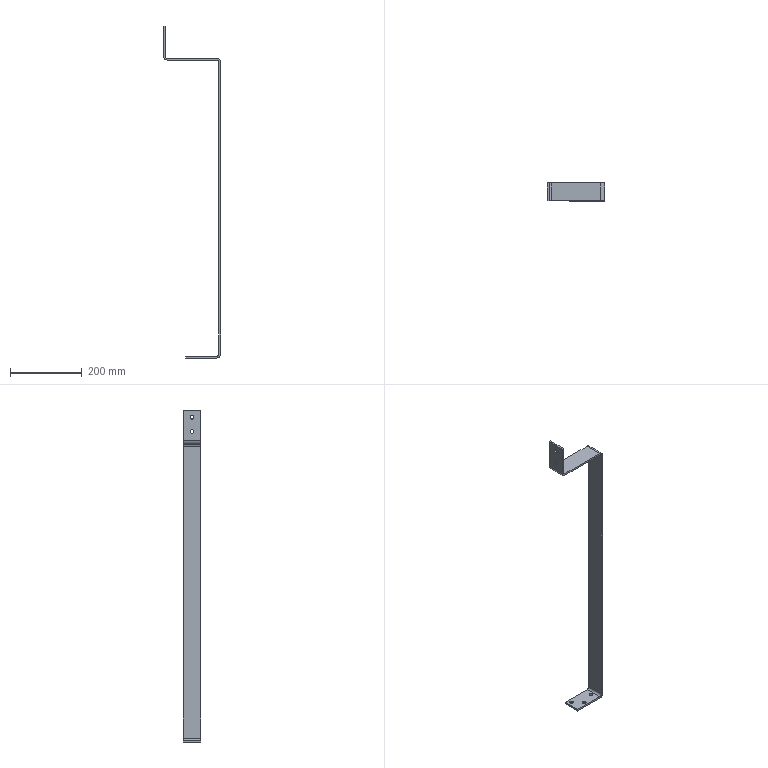Part | SolidWorks | features BaseBody 1 | 1 solid | 28 faces | box 160 x 50 x 926 mm | volume 288422 mm3 | cylinder 16 | plane 12 | commonest cylinder face diameters 11 x8 12 x3 22 x3 10.6 x2
STEP:
#1=CARTESIAN_POINT('',(787.946,-3577.473,1065.971));
#2=VERTEX_POINT('',#1);
#3=CARTESIAN_POINT('',(787.946,-3577.473,1076.971));
#4=VERTEX_POINT('',#3);
#5=CARTESIAN_POINT('',(787.946,-3577.473,1071.471));
#6=DIRECTION('',(-1.,0.,0.));
#7=DIRECTION('',(0.,0.,1.));
#8=AXIS2_PLACEMENT_3D('',#5,#6,#7);
#9=CIRCLE('',#8,5.5);
#10=EDGE_CURVE('',#2,#4,#9,.T.);
#11=ORIENTED_EDGE('',*,*,#10,.F.);
#12=CARTESIAN_POINT('',(782.946,-3577.473,1065.971));
#13=VERTEX_POINT('',#12);
#14=CARTESIAN_POINT('',(781.319,-3577.473,1065.971));
#15=DIRECTION('',(-1.,0.,0.));
#16=VECTOR('',#15,1000.);
#17=LINE('',#14,#16);
#18=EDGE_CURVE('',#2,#13,#17,.T.);
#19=ORIENTED_EDGE('',*,*,#18,.T.);
#20=CARTESIAN_POINT('',(782.946,-3577.473,1076.971));
#21=VERTEX_POINT('',#20);
#22=CARTESIAN_POINT('',(782.946,-3577.473,1071.471));
#23=DIRECTION('',(1.,0.,0.));
#24=DIRECTION('',(0.,0.,1.));
#25=AXIS2_PLACEMENT_3D('',#22,#23,#24);
#26=CIRCLE('',#25,5.5);
#27=EDGE_CURVE('',#21,#13,#26,.T.);
#28=ORIENTED_EDGE('',*,*,#27,.F.);
#29=CARTESIAN_POINT('',(781.319,-3577.473,1076.971));
#30=DIRECTION('',(-1.,0.,0.));
#31=VECTOR('',#30,1000.);
#32=LINE('',#29,#31);
#33=EDGE_CURVE('',#4,#21,#32,.T.);
#34=ORIENTED_EDGE('',*,*,#33,.F.);
#35=EDGE_LOOP('',(#11,#19,#28,#34));
#36=FACE_OUTER_BOUND('',#35,.T.);
#37=CARTESIAN_POINT('',(781.319,-3577.473,1071.471));
#38=DIRECTION('',(-1.,0.,0.));
#39=DIRECTION('',(0.,0.,1.));
#40=AXIS2_PLACEMENT_3D('',#37,#38,#39);
#41=CYLINDRICAL_SURFACE('',#40,5.5);
#42=ADVANCED_FACE('',(#36),#41,.F.);
#43=CARTESIAN_POINT('',(787.946,-3577.473,1025.971));
#44=VERTEX_POINT('',#43);
#45=CARTESIAN_POINT('',(787.946,-3577.473,1036.971));
#46=VERTEX_POINT('',#45);
#47=CARTESIAN_POINT('',(787.946,-3577.473,1031.471));
#48=DIRECTION('',(-1.,0.,0.));
#49=DIRECTION('',(0.,0.,1.));
#50=AXIS2_PLACEMENT_3D('',#47,#48,#49);
#51=CIRCLE('',#50,5.5);
#52=EDGE_CURVE('',#44,#46,#51,.T.);
#53=ORIENTED_EDGE('',*,*,#52,.F.);
#54=CARTESIAN_POINT('',(782.946,-3577.473,1025.971));
#55=VERTEX_POINT('',#54);
#56=CARTESIAN_POINT('',(781.319,-3577.473,1025.971));
#57=DIRECTION('',(-1.,0.,0.));
#58=VECTOR('',#57,1000.);
#59=LINE('',#56,#58);
#60=EDGE_CURVE('',#44,#55,#59,.T.);
#61=ORIENTED_EDGE('',*,*,#60,.T.);
#62=CARTESIAN_POINT('',(782.946,-3577.473,1036.971));
#63=VERTEX_POINT('',#62);
#64=CARTESIAN_POINT('',(782.946,-3577.473,1031.471));
#65=DIRECTION('',(1.,0.,0.));
#66=DIRECTION('',(0.,0.,1.));
#67=AXIS2_PLACEMENT_3D('',#64,#65,#66);
#68=CIRCLE('',#67,5.5);
#69=EDGE_CURVE('',#63,#55,#68,.T.);
#70=ORIENTED_EDGE('',*,*,#69,.F.);
#71=CARTESIAN_POINT('',(781.319,-3577.473,1036.971));
#72=DIRECTION('',(-1.,0.,0.));
#73=VECTOR('',#72,1000.);
#74=LINE('',#71,#73);
#75=EDGE_CURVE('',#46,#63,#74,.T.);
#76=ORIENTED_EDGE('',*,*,#75,.F.);
#77=EDGE_LOOP('',(#53,#61,#70,#76));
#78=FACE_OUTER_BOUND('',#77,.T.);
#79=CARTESIAN_POINT('',(781.319,-3577.473,1031.471));
#80=DIRECTION('',(-1.,0.,0.));
#81=DIRECTION('',(0.,0.,1.));
#82=AXIS2_PLACEMENT_3D('',#79,#80,#81);
#83=CYLINDRICAL_SURFACE('',#82,5.5);
#84=ADVANCED_FACE('',(#78),#83,.F.);
#85=CARTESIAN_POINT('',(916.646,-3577.473,165.471));
#86=VERTEX_POINT('',#85);
#87=CARTESIAN_POINT('',(927.246,-3577.473,165.471));
#88=VERTEX_POINT('',#87);
#89=CARTESIAN_POINT('',(921.946,-3577.473,165.471));
#90=DIRECTION('',(0.,0.,1.));
#91=DIRECTION('',(1.,0.,0.));
#92=AXIS2_PLACEMENT_3D('',#89,#90,#91);
#93=CIRCLE('',#92,5.3);
#94=EDGE_CURVE('',#86,#88,#93,.T.);
#95=ORIENTED_EDGE('',*,*,#94,.F.);
#96=CARTESIAN_POINT('',(916.646,-3577.473,170.471));
#97=VERTEX_POINT('',#96);
#98=CARTESIAN_POINT('',(916.646,-3577.473,155.54));
#99=DIRECTION('',(0.,0.,1.));
#100=VECTOR('',#99,1000.);
#101=LINE('',#98,#100);
#102=EDGE_CURVE('',#86,#97,#101,.T.);
#103=ORIENTED_EDGE('',*,*,#102,.T.);
#104=CARTESIAN_POINT('',(927.246,-3577.473,170.471));
#105=VERTEX_POINT('',#104);
#106=CARTESIAN_POINT('',(921.946,-3577.473,170.471));
#107=DIRECTION('',(0.,0.,-1.));
#108=DIRECTION('',(1.,0.,0.));
#109=AXIS2_PLACEMENT_3D('',#106,#107,#108);
#110=CIRCLE('',#109,5.3);
#111=EDGE_CURVE('',#105,#97,#110,.T.);
#112=ORIENTED_EDGE('',*,*,#111,.F.);
#113=CARTESIAN_POINT('',(927.246,-3577.473,155.54));
#114=DIRECTION('',(0.,0.,1.));
#115=VECTOR('',#114,1000.);
#116=LINE('',#113,#115);
#117=EDGE_CURVE('',#88,#105,#116,.T.);
#118=ORIENTED_EDGE('',*,*,#117,.F.);
#119=EDGE_LOOP('',(#95,#103,#112,#118));
#120=FACE_OUTER_BOUND('',#119,.T.);
#121=CARTESIAN_POINT('',(921.946,-3577.473,155.54));
#122=DIRECTION('',(0.,0.,1.));
#123=DIRECTION('',(1.,0.,0.));
#124=AXIS2_PLACEMENT_3D('',#121,#122,#123);
#125=CYLINDRICAL_SURFACE('',#124,5.3);
#126=ADVANCED_FACE('',(#120),#125,.F.);
#127=CARTESIAN_POINT('',(851.946,-3564.973,165.471));
#128=VERTEX_POINT('',#127);
#129=CARTESIAN_POINT('',(862.946,-3564.973,165.471));
#130=VERTEX_POINT('',#129);
#131=CARTESIAN_POINT('',(857.446,-3564.973,165.471));
#132=DIRECTION('',(0.,0.,1.));
#133=DIRECTION('',(1.,0.,0.));
#134=AXIS2_PLACEMENT_3D('',#131,#132,#133);
#135=CIRCLE('',#134,5.5);
#136=EDGE_CURVE('',#128,#130,#135,.T.);
#137=ORIENTED_EDGE('',*,*,#136,.F.);
#138=CARTESIAN_POINT('',(851.946,-3564.973,170.471));
#139=VERTEX_POINT('',#138);
#140=CARTESIAN_POINT('',(851.946,-3564.973,188.847));
#141=DIRECTION('',(0.,0.,1.));
#142=VECTOR('',#141,1000.);
#143=LINE('',#140,#142);
#144=EDGE_CURVE('',#128,#139,#143,.T.);
#145=ORIENTED_EDGE('',*,*,#144,.T.);
#146=CARTESIAN_POINT('',(862.946,-3564.973,170.471));
#147=VERTEX_POINT('',#146);
#148=CARTESIAN_POINT('',(857.446,-3564.973,170.471));
#149=DIRECTION('',(0.,0.,-1.));
#150=DIRECTION('',(1.,0.,0.));
#151=AXIS2_PLACEMENT_3D('',#148,#149,#150);
#152=CIRCLE('',#151,5.5);
#153=EDGE_CURVE('',#147,#139,#152,.T.);
#154=ORIENTED_EDGE('',*,*,#153,.F.);
#155=CARTESIAN_POINT('',(862.946,-3564.973,188.847));
#156=DIRECTION('',(0.,0.,1.));
#157=VECTOR('',#156,1000.);
#158=LINE('',#155,#157);
#159=EDGE_CURVE('',#130,#147,#158,.T.);
#160=ORIENTED_EDGE('',*,*,#159,.F.);
#161=EDGE_LOOP('',(#137,#145,#154,#160));
#162=FACE_OUTER_BOUND('',#161,.T.);
#163=CARTESIAN_POINT('',(857.446,-3564.973,188.847));
#164=DIRECTION('',(0.,0.,1.));
#165=DIRECTION('',(1.,0.,0.));
#166=AXIS2_PLACEMENT_3D('',#163,#164,#165);
#167=CYLINDRICAL_SURFACE('',#166,5.5);
#168=ADVANCED_FACE('',(#162),#167,.F.);
#169=CARTESIAN_POINT('',(887.946,-3589.973,170.471));
#170=VERTEX_POINT('',#169);
#171=CARTESIAN_POINT('',(876.946,-3589.973,170.471));
#172=VERTEX_POINT('',#171);
#173=CARTESIAN_POINT('',(882.446,-3589.973,170.471));
#174=DIRECTION('',(0.,0.,-1.));
#175=DIRECTION('',(-1.,0.,0.));
#176=AXIS2_PLACEMENT_3D('',#173,#174,#175);
#177=CIRCLE('',#176,5.5);
#178=EDGE_CURVE('',#170,#172,#177,.T.);
#179=ORIENTED_EDGE('',*,*,#178,.F.);
#180=CARTESIAN_POINT('',(887.946,-3589.973,165.471));
#181=VERTEX_POINT('',#180);
#182=CARTESIAN_POINT('',(887.946,-3589.973,188.847));
#183=DIRECTION('',(0.,0.,-1.));
#184=VECTOR('',#183,1000.);
#185=LINE('',#182,#184);
#186=EDGE_CURVE('',#170,#181,#185,.T.);
#187=ORIENTED_EDGE('',*,*,#186,.T.);
#188=CARTESIAN_POINT('',(876.946,-3589.973,165.471));
#189=VERTEX_POINT('',#188);
#190=CARTESIAN_POINT('',(882.446,-3589.973,165.471));
#191=DIRECTION('',(0.,0.,1.));
#192=DIRECTION('',(-1.,0.,0.));
#193=AXIS2_PLACEMENT_3D('',#190,#191,#192);
#194=CIRCLE('',#193,5.5);
#195=EDGE_CURVE('',#189,#181,#194,.T.);
#196=ORIENTED_EDGE('',*,*,#195,.F.);
#197=CARTESIAN_POINT('',(876.946,-3589.973,188.847));
#198=DIRECTION('',(0.,0.,-1.));
#199=VECTOR('',#198,1000.);
#200=LINE('',#197,#199);
#201=EDGE_CURVE('',#172,#189,#200,.T.);
#202=ORIENTED_EDGE('',*,*,#201,.F.);
#203=EDGE_LOOP('',(#179,#187,#196,#202));
#204=FACE_OUTER_BOUND('',#203,.T.);
#205=CARTESIAN_POINT('',(882.446,-3589.973,188.847));
#206=DIRECTION('',(0.,0.,-1.));
#207=DIRECTION('',(-1.,0.,0.));
#208=AXIS2_PLACEMENT_3D('',#205,#206,#207);
#209=CYLINDRICAL_SURFACE('',#208,5.5);
#210=ADVANCED_FACE('',(#204),#209,.F.);
#211=CARTESIAN_POINT('',(942.946,-3552.473,176.471));
#212=VERTEX_POINT('',#211);
#213=CARTESIAN_POINT('',(942.946,-3552.473,990.471));
#214=VERTEX_POINT('',#213);
#215=CARTESIAN_POINT('',(942.946,-3552.473,990.471));
#216=DIRECTION('',(0.,0.,1.));
#217=VECTOR('',#216,1000.);
#218=LINE('',#215,#217);
#219=EDGE_CURVE('',#212,#214,#218,.T.);
#220=ORIENTED_EDGE('',*,*,#219,.T.);
#221=CARTESIAN_POINT('',(942.946,-3602.473,990.471));
#222=VERTEX_POINT('',#221);
#223=CARTESIAN_POINT('',(942.946,-3552.473,990.471));
#224=DIRECTION('',(0.,-1.,0.));
#225=VECTOR('',#224,1000.);
#226=LINE('',#223,#225);
#227=EDGE_CURVE('',#214,#222,#226,.T.);
#228=ORIENTED_EDGE('',*,*,#227,.T.);
#229=CARTESIAN_POINT('',(942.946,-3602.473,176.471));
#230=VERTEX_POINT('',#229);
#231=CARTESIAN_POINT('',(942.946,-3602.473,990.471));
#232=DIRECTION('',(0.,0.,-1.));
#233=VECTOR('',#232,1000.);
#234=LINE('',#231,#233);
#235=EDGE_CURVE('',#222,#230,#234,.T.);
#236=ORIENTED_EDGE('',*,*,#235,.T.);
#237=CARTESIAN_POINT('',(942.946,-3552.473,176.471));
#238=DIRECTION('',(0.,1.,0.));
#239=VECTOR('',#238,1000.);
#240=LINE('',#237,#239);
#241=EDGE_CURVE('',#230,#212,#240,.T.);
#242=ORIENTED_EDGE('',*,*,#241,.T.);
#243=EDGE_LOOP('',(#220,#228,#236,#242));
#244=FACE_OUTER_BOUND('',#243,.T.);
#245=CARTESIAN_POINT('',(942.946,-3552.473,990.471));
#246=DIRECTION('',(1.,0.,0.));
#247=DIRECTION('',(0.,1.,0.));
#248=AXIS2_PLACEMENT_3D('',#245,#246,#247);
#249=PLANE('',#248);
#250=ADVANCED_FACE('',(#244),#249,.T.);
#251=CARTESIAN_POINT('',(931.946,-3552.473,1001.471));
#252=VERTEX_POINT('',#251);
#253=CARTESIAN_POINT('',(931.946,-3552.473,990.471));
#254=DIRECTION('',(0.,-1.,0.));
#255=DIRECTION('',(0.,0.,-1.));
#256=AXIS2_PLACEMENT_3D('',#253,#254,#255);
#257=CIRCLE('',#256,11.);
#258=EDGE_CURVE('',#214,#252,#257,.T.);
#259=ORIENTED_EDGE('',*,*,#258,.T.);
#260=CARTESIAN_POINT('',(931.946,-3602.473,1001.471));
#261=VERTEX_POINT('',#260);
#262=CARTESIAN_POINT('',(931.946,-3552.473,1001.471));
#263=DIRECTION('',(0.,-1.,0.));
#264=VECTOR('',#263,1000.);
#265=LINE('',#262,#264);
#266=EDGE_CURVE('',#252,#261,#265,.T.);
#267=ORIENTED_EDGE('',*,*,#266,.T.);
#268=CARTESIAN_POINT('',(931.946,-3602.473,990.471));
#269=DIRECTION('',(0.,1.,0.));
#270=DIRECTION('',(0.,0.,-1.));
#271=AXIS2_PLACEMENT_3D('',#268,#269,#270);
#272=CIRCLE('',#271,11.);
#273=EDGE_CURVE('',#261,#222,#272,.T.);
#274=ORIENTED_EDGE('',*,*,#273,.T.);
#275=ORIENTED_EDGE('',*,*,#227,.F.);
#276=EDGE_LOOP('',(#259,#267,#274,#275));
#277=FACE_OUTER_BOUND('',#276,.T.);
#278=CARTESIAN_POINT('',(931.946,-3552.473,990.471));
#279=DIRECTION('',(0.,-1.,0.));
#280=DIRECTION('',(0.,0.,-1.));
#281=AXIS2_PLACEMENT_3D('',#278,#279,#280);
#282=CYLINDRICAL_SURFACE('',#281,11.);
#283=ADVANCED_FACE('',(#277),#282,.T.);
#284=ORIENTED_EDGE('',*,*,#258,.F.);
#285=ORIENTED_EDGE('',*,*,#219,.F.);
#286=CARTESIAN_POINT('',(931.946,-3552.473,165.471));
#287=VERTEX_POINT('',#286);
#288=CARTESIAN_POINT('',(931.946,-3552.473,176.471));
#289=DIRECTION('',(0.,1.,0.));
#290=DIRECTION('',(0.,0.,-1.));
#291=AXIS2_PLACEMENT_3D('',#288,#289,#290);
#292=CIRCLE('',#291,11.);
#293=EDGE_CURVE('',#212,#287,#292,.T.);
#294=ORIENTED_EDGE('',*,*,#293,.T.);
#295=CARTESIAN_POINT('',(844.946,-3552.473,165.471));
#296=VERTEX_POINT('',#295);
#297=CARTESIAN_POINT('',(913.142,-3552.473,165.471));
#298=DIRECTION('',(-1.,0.,0.));
#299=VECTOR('',#298,1000.);
#300=LINE('',#297,#299);
#301=EDGE_CURVE('',#287,#296,#300,.T.);
#302=ORIENTED_EDGE('',*,*,#301,.T.);
#303=CARTESIAN_POINT('',(844.946,-3552.473,170.471));
#304=VERTEX_POINT('',#303);
#305=CARTESIAN_POINT('',(844.946,-3552.473,635.303));
#306=DIRECTION('',(0.,0.,1.));
#307=VECTOR('',#306,1000.);
#308=LINE('',#305,#307);
#309=EDGE_CURVE('',#296,#304,#308,.T.);
#310=ORIENTED_EDGE('',*,*,#309,.T.);
#311=CARTESIAN_POINT('',(931.946,-3552.473,170.471));
#312=VERTEX_POINT('',#311);
#313=CARTESIAN_POINT('',(913.142,-3552.473,170.471));
#314=DIRECTION('',(1.,0.,0.));
#315=VECTOR('',#314,1000.);
#316=LINE('',#313,#315);
#317=EDGE_CURVE('',#304,#312,#316,.T.);
#318=ORIENTED_EDGE('',*,*,#317,.T.);
#319=CARTESIAN_POINT('',(937.946,-3552.473,176.471));
#320=VERTEX_POINT('',#319);
#321=CARTESIAN_POINT('',(931.946,-3552.473,176.471));
#322=DIRECTION('',(0.,-1.,0.));
#323=DIRECTION('',(0.,0.,-1.));
#324=AXIS2_PLACEMENT_3D('',#321,#322,#323);
#325=CIRCLE('',#324,6.);
#326=EDGE_CURVE('',#312,#320,#325,.T.);
#327=ORIENTED_EDGE('',*,*,#326,.T.);
#328=CARTESIAN_POINT('',(937.946,-3552.473,990.471));
#329=VERTEX_POINT('',#328);
#330=CARTESIAN_POINT('',(937.946,-3552.473,635.303));
#331=DIRECTION('',(0.,0.,1.));
#332=VECTOR('',#331,1000.);
#333=LINE('',#330,#332);
#334=EDGE_CURVE('',#320,#329,#333,.T.);
#335=ORIENTED_EDGE('',*,*,#334,.T.);
#336=CARTESIAN_POINT('',(931.946,-3552.473,996.471));
#337=VERTEX_POINT('',#336);
#338=CARTESIAN_POINT('',(931.946,-3552.473,990.471));
#339=DIRECTION('',(0.,-1.,0.));
#340=DIRECTION('',(0.,0.,-1.));
#341=AXIS2_PLACEMENT_3D('',#338,#339,#340);
#342=CIRCLE('',#341,6.);
#343=EDGE_CURVE('',#329,#337,#342,.T.);
#344=ORIENTED_EDGE('',*,*,#343,.T.);
#345=CARTESIAN_POINT('',(793.946,-3552.473,996.471));
#346=VERTEX_POINT('',#345);
#347=CARTESIAN_POINT('',(913.142,-3552.473,996.471));
#348=DIRECTION('',(-1.,0.,0.));
#349=VECTOR('',#348,1000.);
#350=LINE('',#347,#349);
#351=EDGE_CURVE('',#337,#346,#350,.T.);
#352=ORIENTED_EDGE('',*,*,#351,.T.);
#353=CARTESIAN_POINT('',(782.946,-3552.473,1007.471));
#354=VERTEX_POINT('',#353);
#355=CARTESIAN_POINT('',(793.946,-3552.473,1007.471));
#356=DIRECTION('',(0.,1.,0.));
#357=DIRECTION('',(0.,0.,-1.));
#358=AXIS2_PLACEMENT_3D('',#355,#356,#357);
#359=CIRCLE('',#358,11.);
#360=EDGE_CURVE('',#346,#354,#359,.T.);
#361=ORIENTED_EDGE('',*,*,#360,.T.);
#362=CARTESIAN_POINT('',(782.946,-3552.473,1091.471));
#363=VERTEX_POINT('',#362);
#364=CARTESIAN_POINT('',(782.946,-3552.473,635.303));
#365=DIRECTION('',(0.,0.,1.));
#366=VECTOR('',#365,1000.);
#367=LINE('',#364,#366);
#368=EDGE_CURVE('',#354,#363,#367,.T.);
#369=ORIENTED_EDGE('',*,*,#368,.T.);
#370=CARTESIAN_POINT('',(787.946,-3552.473,1091.471));
#371=VERTEX_POINT('',#370);
#372=CARTESIAN_POINT('',(913.142,-3552.473,1091.471));
#373=DIRECTION('',(1.,0.,0.));
#374=VECTOR('',#373,1000.);
#375=LINE('',#372,#374);
#376=EDGE_CURVE('',#363,#371,#375,.T.);
#377=ORIENTED_EDGE('',*,*,#376,.T.);
#378=CARTESIAN_POINT('',(787.946,-3552.473,1007.471));
#379=VERTEX_POINT('',#378);
#380=CARTESIAN_POINT('',(787.946,-3552.473,635.303));
#381=DIRECTION('',(0.,0.,-1.));
#382=VECTOR('',#381,1000.);
#383=LINE('',#380,#382);
#384=EDGE_CURVE('',#371,#379,#383,.T.);
#385=ORIENTED_EDGE('',*,*,#384,.T.);
#386=CARTESIAN_POINT('',(793.946,-3552.473,1001.471));
#387=VERTEX_POINT('',#386);
#388=CARTESIAN_POINT('',(793.946,-3552.473,1007.471));
#389=DIRECTION('',(0.,-1.,0.));
#390=DIRECTION('',(0.,0.,-1.));
#391=AXIS2_PLACEMENT_3D('',#388,#389,#390);
#392=CIRCLE('',#391,6.);
#393=EDGE_CURVE('',#379,#387,#392,.T.);
#394=ORIENTED_EDGE('',*,*,#393,.T.);
#395=CARTESIAN_POINT('',(913.142,-3552.473,1001.471));
#396=DIRECTION('',(1.,0.,0.));
#397=VECTOR('',#396,1000.);
#398=LINE('',#395,#397);
#399=EDGE_CURVE('',#387,#252,#398,.T.);
#400=ORIENTED_EDGE('',*,*,#399,.T.);
#401=EDGE_LOOP('',(#284,#285,#294,#302,#310,#318,#327,#335,#344,#352,#361,#369,#377,#385,#394,#400));
#402=FACE_OUTER_BOUND('',#401,.T.);
#403=CARTESIAN_POINT('',(913.142,-3552.473,635.303));
#404=DIRECTION('',(0.,1.,0.));
#405=DIRECTION('',(0.,0.,1.));
#406=AXIS2_PLACEMENT_3D('',#403,#404,#405);
#407=PLANE('',#406);
#408=ADVANCED_FACE('',(#402),#407,.T.);
#409=ORIENTED_EDGE('',*,*,#293,.F.);
#410=ORIENTED_EDGE('',*,*,#241,.F.);
#411=CARTESIAN_POINT('',(931.946,-3602.473,165.471));
#412=VERTEX_POINT('',#411);
#413=CARTESIAN_POINT('',(931.946,-3602.473,176.471));
#414=DIRECTION('',(0.,1.,0.));
#415=DIRECTION('',(0.,0.,-1.));
#416=AXIS2_PLACEMENT_3D('',#413,#414,#415);
#417=CIRCLE('',#416,11.);
#418=EDGE_CURVE('',#230,#412,#417,.T.);
#419=ORIENTED_EDGE('',*,*,#418,.T.);
#420=CARTESIAN_POINT('',(931.946,-3552.473,165.471));
#421=DIRECTION('',(0.,1.,0.));
#422=VECTOR('',#421,1000.);
#423=LINE('',#420,#422);
#424=EDGE_CURVE('',#412,#287,#423,.T.);
#425=ORIENTED_EDGE('',*,*,#424,.T.);
#426=EDGE_LOOP('',(#409,#410,#419,#425));
#427=FACE_OUTER_BOUND('',#426,.T.);
#428=CARTESIAN_POINT('',(931.946,-3552.473,176.471));
#429=DIRECTION('',(0.,-1.,0.));
#430=DIRECTION('',(0.,0.,-1.));
#431=AXIS2_PLACEMENT_3D('',#428,#429,#430);
#432=CYLINDRICAL_SURFACE('',#431,11.);
#433=ADVANCED_FACE('',(#427),#432,.T.);
#434=ORIENTED_EDGE('',*,*,#418,.F.);
#435=ORIENTED_EDGE('',*,*,#235,.F.);
#436=ORIENTED_EDGE('',*,*,#273,.F.);
#437=CARTESIAN_POINT('',(793.946,-3602.473,1001.471));
#438=VERTEX_POINT('',#437);
#439=CARTESIAN_POINT('',(913.142,-3602.473,1001.471));
#440=DIRECTION('',(1.,0.,0.));
#441=VECTOR('',#440,1000.);
#442=LINE('',#439,#441);
#443=EDGE_CURVE('',#438,#261,#442,.T.);
#444=ORIENTED_EDGE('',*,*,#443,.F.);
#445=CARTESIAN_POINT('',(787.946,-3602.473,1007.471));
#446=VERTEX_POINT('',#445);
#447=CARTESIAN_POINT('',(793.946,-3602.473,1007.471));
#448=DIRECTION('',(0.,-1.,0.));
#449=DIRECTION('',(0.,0.,-1.));
#450=AXIS2_PLACEMENT_3D('',#447,#448,#449);
#451=CIRCLE('',#450,6.);
#452=EDGE_CURVE('',#446,#438,#451,.T.);
#453=ORIENTED_EDGE('',*,*,#452,.F.);
#454=CARTESIAN_POINT('',(787.946,-3602.473,1091.471));
#455=VERTEX_POINT('',#454);
#456=CARTESIAN_POINT('',(787.946,-3602.473,635.303));
#457=DIRECTION('',(0.,0.,-1.));
#458=VECTOR('',#457,1000.);
#459=LINE('',#456,#458);
#460=EDGE_CURVE('',#455,#446,#459,.T.);
#461=ORIENTED_EDGE('',*,*,#460,.F.);
#462=CARTESIAN_POINT('',(782.946,-3602.473,1091.471));
#463=VERTEX_POINT('',#462);
#464=CARTESIAN_POINT('',(913.142,-3602.473,1091.471));
#465=DIRECTION('',(1.,0.,0.));
#466=VECTOR('',#465,1000.);
#467=LINE('',#464,#466);
#468=EDGE_CURVE('',#463,#455,#467,.T.);
#469=ORIENTED_EDGE('',*,*,#468,.F.);
#470=CARTESIAN_POINT('',(782.946,-3602.473,1007.471));
#471=VERTEX_POINT('',#470);
#472=CARTESIAN_POINT('',(782.946,-3602.473,635.303));
#473=DIRECTION('',(0.,0.,1.));
#474=VECTOR('',#473,1000.);
#475=LINE('',#472,#474);
#476=EDGE_CURVE('',#471,#463,#475,.T.);
#477=ORIENTED_EDGE('',*,*,#476,.F.);
#478=CARTESIAN_POINT('',(793.946,-3602.473,996.471));
#479=VERTEX_POINT('',#478);
#480=CARTESIAN_POINT('',(793.946,-3602.473,1007.471));
#481=DIRECTION('',(0.,1.,0.));
#482=DIRECTION('',(0.,0.,-1.));
#483=AXIS2_PLACEMENT_3D('',#480,#481,#482);
#484=CIRCLE('',#483,11.);
#485=EDGE_CURVE('',#479,#471,#484,.T.);
#486=ORIENTED_EDGE('',*,*,#485,.F.);
#487=CARTESIAN_POINT('',(931.946,-3602.473,996.471));
#488=VERTEX_POINT('',#487);
#489=CARTESIAN_POINT('',(913.142,-3602.473,996.471));
#490=DIRECTION('',(-1.,0.,0.));
#491=VECTOR('',#490,1000.);
#492=LINE('',#489,#491);
#493=EDGE_CURVE('',#488,#479,#492,.T.);
#494=ORIENTED_EDGE('',*,*,#493,.F.);
#495=CARTESIAN_POINT('',(937.946,-3602.473,990.471));
#496=VERTEX_POINT('',#495);
#497=CARTESIAN_POINT('',(931.946,-3602.473,990.471));
#498=DIRECTION('',(0.,-1.,0.));
#499=DIRECTION('',(0.,0.,-1.));
#500=AXIS2_PLACEMENT_3D('',#497,#498,#499);
#501=CIRCLE('',#500,6.);
#502=EDGE_CURVE('',#496,#488,#501,.T.);
#503=ORIENTED_EDGE('',*,*,#502,.F.);
#504=CARTESIAN_POINT('',(937.946,-3602.473,176.471));
#505=VERTEX_POINT('',#504);
#506=CARTESIAN_POINT('',(937.946,-3602.473,635.303));
#507=DIRECTION('',(0.,0.,1.));
#508=VECTOR('',#507,1000.);
#509=LINE('',#506,#508);
#510=EDGE_CURVE('',#505,#496,#509,.T.);
#511=ORIENTED_EDGE('',*,*,#510,.F.);
#512=CARTESIAN_POINT('',(931.946,-3602.473,170.471));
#513=VERTEX_POINT('',#512);
#514=CARTESIAN_POINT('',(931.946,-3602.473,176.471));
#515=DIRECTION('',(0.,-1.,0.));
#516=DIRECTION('',(0.,0.,-1.));
#517=AXIS2_PLACEMENT_3D('',#514,#515,#516);
#518=CIRCLE('',#517,6.);
#519=EDGE_CURVE('',#513,#505,#518,.T.);
#520=ORIENTED_EDGE('',*,*,#519,.F.);
#521=CARTESIAN_POINT('',(844.946,-3602.473,170.471));
#522=VERTEX_POINT('',#521);
#523=CARTESIAN_POINT('',(913.142,-3602.473,170.471));
#524=DIRECTION('',(1.,0.,0.));
#525=VECTOR('',#524,1000.);
#526=LINE('',#523,#525);
#527=EDGE_CURVE('',#522,#513,#526,.T.);
#528=ORIENTED_EDGE('',*,*,#527,.F.);
#529=CARTESIAN_POINT('',(844.946,-3602.473,165.471));
#530=VERTEX_POINT('',#529);
#531=CARTESIAN_POINT('',(844.946,-3602.473,635.303));
#532=DIRECTION('',(0.,0.,1.));
#533=VECTOR('',#532,1000.);
#534=LINE('',#531,#533);
#535=EDGE_CURVE('',#530,#522,#534,.T.);
#536=ORIENTED_EDGE('',*,*,#535,.F.);
#537=CARTESIAN_POINT('',(913.142,-3602.473,165.471));
#538=DIRECTION('',(-1.,0.,0.));
#539=VECTOR('',#538,1000.);
#540=LINE('',#537,#539);
#541=EDGE_CURVE('',#412,#530,#540,.T.);
#542=ORIENTED_EDGE('',*,*,#541,.F.);
#543=EDGE_LOOP('',(#434,#435,#436,#444,#453,#461,#469,#477,#486,#494,#503,#511,#520,#528,#536,#542));
#544=FACE_OUTER_BOUND('',#543,.T.);
#545=CARTESIAN_POINT('',(913.142,-3602.473,635.303));
#546=DIRECTION('',(0.,1.,0.));
#547=DIRECTION('',(0.,0.,1.));
#548=AXIS2_PLACEMENT_3D('',#545,#546,#547);
#549=PLANE('',#548);
#550=ADVANCED_FACE('',(#544),#549,.F.);
#551=ORIENTED_EDGE('',*,*,#399,.F.);
#552=CARTESIAN_POINT('',(793.946,-3552.473,1001.471));
#553=DIRECTION('',(0.,-1.,0.));
#554=VECTOR('',#553,1000.);
#555=LINE('',#552,#554);
#556=EDGE_CURVE('',#387,#438,#555,.T.);
#557=ORIENTED_EDGE('',*,*,#556,.T.);
#558=ORIENTED_EDGE('',*,*,#443,.T.);
#559=ORIENTED_EDGE('',*,*,#266,.F.);
#560=EDGE_LOOP('',(#551,#557,#558,#559));
#561=FACE_OUTER_BOUND('',#560,.T.);
#562=CARTESIAN_POINT('',(793.946,-3552.473,1001.471));
#563=DIRECTION('',(0.,0.,1.));
#564=DIRECTION('',(0.,-1.,0.));
#565=AXIS2_PLACEMENT_3D('',#562,#563,#564);
#566=PLANE('',#565);
#567=ADVANCED_FACE('',(#561),#566,.T.);
#568=ORIENTED_EDGE('',*,*,#393,.F.);
#569=CARTESIAN_POINT('',(787.946,-3552.473,1007.471));
#570=DIRECTION('',(0.,-1.,0.));
#571=VECTOR('',#570,1000.);
#572=LINE('',#569,#571);
#573=EDGE_CURVE('',#379,#446,#572,.T.);
#574=ORIENTED_EDGE('',*,*,#573,.T.);
#575=ORIENTED_EDGE('',*,*,#452,.T.);
#576=ORIENTED_EDGE('',*,*,#556,.F.);
#577=EDGE_LOOP('',(#568,#574,#575,#576));
#578=FACE_OUTER_BOUND('',#577,.T.);
#579=CARTESIAN_POINT('',(793.946,-3552.473,1007.471));
#580=DIRECTION('',(0.,-1.,0.));
#581=DIRECTION('',(0.,0.,-1.));
#582=AXIS2_PLACEMENT_3D('',#579,#580,#581);
#583=CYLINDRICAL_SURFACE('',#582,6.);
#584=ADVANCED_FACE('',(#578),#583,.F.);
#585=ORIENTED_EDGE('',*,*,#384,.F.);
#586=CARTESIAN_POINT('',(787.946,-3552.473,1091.471));
#587=DIRECTION('',(0.,-1.,0.));
#588=VECTOR('',#587,1000.);
#589=LINE('',#586,#588);
#590=EDGE_CURVE('',#371,#455,#589,.T.);
#591=ORIENTED_EDGE('',*,*,#590,.T.);
#592=ORIENTED_EDGE('',*,*,#460,.T.);
#593=ORIENTED_EDGE('',*,*,#573,.F.);
#594=EDGE_LOOP('',(#585,#591,#592,#593));
#595=FACE_OUTER_BOUND('',#594,.T.);
#596=CARTESIAN_POINT('',(787.946,-3577.473,1071.471));
#597=DIRECTION('',(-1.,0.,0.));
#598=DIRECTION('',(0.,0.,1.));
#599=AXIS2_PLACEMENT_3D('',#596,#597,#598);
#600=CIRCLE('',#599,5.5);
#601=EDGE_CURVE('',#4,#2,#600,.T.);
#602=ORIENTED_EDGE('',*,*,#601,.T.);
#603=ORIENTED_EDGE('',*,*,#10,.T.);
#604=EDGE_LOOP('',(#602,#603));
#605=FACE_BOUND('',#604,.T.);
#606=CARTESIAN_POINT('',(787.946,-3577.473,1031.471));
#607=DIRECTION('',(-1.,0.,0.));
#608=DIRECTION('',(0.,0.,1.));
#609=AXIS2_PLACEMENT_3D('',#606,#607,#608);
#610=CIRCLE('',#609,5.5);
#611=EDGE_CURVE('',#46,#44,#610,.T.);
#612=ORIENTED_EDGE('',*,*,#611,.T.);
#613=ORIENTED_EDGE('',*,*,#52,.T.);
#614=EDGE_LOOP('',(#612,#613));
#615=FACE_BOUND('',#614,.T.);
#616=CARTESIAN_POINT('',(787.946,-3552.473,1091.471));
#617=DIRECTION('',(1.,0.,0.));
#618=DIRECTION('',(0.,0.,-1.));
#619=AXIS2_PLACEMENT_3D('',#616,#617,#618);
#620=PLANE('',#619);
#621=ADVANCED_FACE('',(#595,#605,#615),#620,.T.);
#622=ORIENTED_EDGE('',*,*,#376,.F.);
#623=CARTESIAN_POINT('',(782.946,-3552.473,1091.471));
#624=DIRECTION('',(0.,-1.,0.));
#625=VECTOR('',#624,1000.);
#626=LINE('',#623,#625);
#627=EDGE_CURVE('',#363,#463,#626,.T.);
#628=ORIENTED_EDGE('',*,*,#627,.T.);
#629=ORIENTED_EDGE('',*,*,#468,.T.);
#630=ORIENTED_EDGE('',*,*,#590,.F.);
#631=EDGE_LOOP('',(#622,#628,#629,#630));
#632=FACE_OUTER_BOUND('',#631,.T.);
#633=CARTESIAN_POINT('',(782.946,-3552.473,1091.471));
#634=DIRECTION('',(0.,0.,1.));
#635=DIRECTION('',(1.,0.,0.));
#636=AXIS2_PLACEMENT_3D('',#633,#634,#635);
#637=PLANE('',#636);
#638=ADVANCED_FACE('',(#632),#637,.T.);
#639=ORIENTED_EDGE('',*,*,#368,.F.);
#640=CARTESIAN_POINT('',(782.946,-3552.473,1007.471));
#641=DIRECTION('',(0.,-1.,0.));
#642=VECTOR('',#641,1000.);
#643=LINE('',#640,#642);
#644=EDGE_CURVE('',#354,#471,#643,.T.);
#645=ORIENTED_EDGE('',*,*,#644,.T.);
#646=ORIENTED_EDGE('',*,*,#476,.T.);
#647=ORIENTED_EDGE('',*,*,#627,.F.);
#648=EDGE_LOOP('',(#639,#645,#646,#647));
#649=FACE_OUTER_BOUND('',#648,.T.);
#650=ORIENTED_EDGE('',*,*,#27,.T.);
#651=CARTESIAN_POINT('',(782.946,-3577.473,1071.471));
#652=DIRECTION('',(1.,0.,0.));
#653=DIRECTION('',(0.,0.,1.));
#654=AXIS2_PLACEMENT_3D('',#651,#652,#653);
#655=CIRCLE('',#654,5.5);
#656=EDGE_CURVE('',#13,#21,#655,.T.);
#657=ORIENTED_EDGE('',*,*,#656,.T.);
#658=EDGE_LOOP('',(#650,#657));
#659=FACE_BOUND('',#658,.T.);
#660=ORIENTED_EDGE('',*,*,#69,.T.);
#661=CARTESIAN_POINT('',(782.946,-3577.473,1031.471));
#662=DIRECTION('',(1.,0.,0.));
#663=DIRECTION('',(0.,0.,1.));
#664=AXIS2_PLACEMENT_3D('',#661,#662,#663);
#665=CIRCLE('',#664,5.5);
#666=EDGE_CURVE('',#55,#63,#665,.T.);
#667=ORIENTED_EDGE('',*,*,#666,.T.);
#668=EDGE_LOOP('',(#660,#667));
#669=FACE_BOUND('',#668,.T.);
#670=CARTESIAN_POINT('',(782.946,-3552.473,1007.471));
#671=DIRECTION('',(-1.,0.,0.));
#672=DIRECTION('',(0.,0.,1.));
#673=AXIS2_PLACEMENT_3D('',#670,#671,#672);
#674=PLANE('',#673);
#675=ADVANCED_FACE('',(#649,#659,#669),#674,.T.);
#676=ORIENTED_EDGE('',*,*,#360,.F.);
#677=CARTESIAN_POINT('',(793.946,-3552.473,996.471));
#678=DIRECTION('',(0.,-1.,0.));
#679=VECTOR('',#678,1000.);
#680=LINE('',#677,#679);
#681=EDGE_CURVE('',#346,#479,#680,.T.);
#682=ORIENTED_EDGE('',*,*,#681,.T.);
#683=ORIENTED_EDGE('',*,*,#485,.T.);
#684=ORIENTED_EDGE('',*,*,#644,.F.);
#685=EDGE_LOOP('',(#676,#682,#683,#684));
#686=FACE_OUTER_BOUND('',#685,.T.);
#687=CARTESIAN_POINT('',(793.946,-3552.473,1007.471));
#688=DIRECTION('',(0.,-1.,0.));
#689=DIRECTION('',(0.,0.,-1.));
#690=AXIS2_PLACEMENT_3D('',#687,#688,#689);
#691=CYLINDRICAL_SURFACE('',#690,11.);
#692=ADVANCED_FACE('',(#686),#691,.T.);
#693=ORIENTED_EDGE('',*,*,#351,.F.);
#694=CARTESIAN_POINT('',(931.946,-3552.473,996.471));
#695=DIRECTION('',(0.,-1.,0.));
#696=VECTOR('',#695,1000.);
#697=LINE('',#694,#696);
#698=EDGE_CURVE('',#337,#488,#697,.T.);
#699=ORIENTED_EDGE('',*,*,#698,.T.);
#700=ORIENTED_EDGE('',*,*,#493,.T.);
#701=ORIENTED_EDGE('',*,*,#681,.F.);
#702=EDGE_LOOP('',(#693,#699,#700,#701));
#703=FACE_OUTER_BOUND('',#702,.T.);
#704=CARTESIAN_POINT('',(931.946,-3552.473,996.471));
#705=DIRECTION('',(0.,0.,-1.));
#706=DIRECTION('',(-1.,0.,0.));
#707=AXIS2_PLACEMENT_3D('',#704,#705,#706);
#708=PLANE('',#707);
#709=ADVANCED_FACE('',(#703),#708,.T.);
#710=ORIENTED_EDGE('',*,*,#343,.F.);
#711=CARTESIAN_POINT('',(937.946,-3552.473,990.471));
#712=DIRECTION('',(0.,-1.,0.));
#713=VECTOR('',#712,1000.);
#714=LINE('',#711,#713);
#715=EDGE_CURVE('',#329,#496,#714,.T.);
#716=ORIENTED_EDGE('',*,*,#715,.T.);
#717=ORIENTED_EDGE('',*,*,#502,.T.);
#718=ORIENTED_EDGE('',*,*,#698,.F.);
#719=EDGE_LOOP('',(#710,#716,#717,#718));
#720=FACE_OUTER_BOUND('',#719,.T.);
#721=CARTESIAN_POINT('',(931.946,-3552.473,990.471));
#722=DIRECTION('',(0.,-1.,0.));
#723=DIRECTION('',(0.,0.,-1.));
#724=AXIS2_PLACEMENT_3D('',#721,#722,#723);
#725=CYLINDRICAL_SURFACE('',#724,6.);
#726=ADVANCED_FACE('',(#720),#725,.F.);
#727=ORIENTED_EDGE('',*,*,#334,.F.);
#728=CARTESIAN_POINT('',(937.946,-3552.473,176.471));
#729=DIRECTION('',(0.,-1.,0.));
#730=VECTOR('',#729,1000.);
#731=LINE('',#728,#730);
#732=EDGE_CURVE('',#320,#505,#731,.T.);
#733=ORIENTED_EDGE('',*,*,#732,.T.);
#734=ORIENTED_EDGE('',*,*,#510,.T.);
#735=ORIENTED_EDGE('',*,*,#715,.F.);
#736=EDGE_LOOP('',(#727,#733,#734,#735));
#737=FACE_OUTER_BOUND('',#736,.T.);
#738=CARTESIAN_POINT('',(937.946,-3552.473,176.471));
#739=DIRECTION('',(-1.,0.,0.));
#740=DIRECTION('',(0.,0.,1.));
#741=AXIS2_PLACEMENT_3D('',#738,#739,#740);
#742=PLANE('',#741);
#743=ADVANCED_FACE('',(#737),#742,.T.);
#744=ORIENTED_EDGE('',*,*,#326,.F.);
#745=CARTESIAN_POINT('',(931.946,-3552.473,170.471));
#746=DIRECTION('',(0.,-1.,0.));
#747=VECTOR('',#746,1000.);
#748=LINE('',#745,#747);
#749=EDGE_CURVE('',#312,#513,#748,.T.);
#750=ORIENTED_EDGE('',*,*,#749,.T.);
#751=ORIENTED_EDGE('',*,*,#519,.T.);
#752=ORIENTED_EDGE('',*,*,#732,.F.);
#753=EDGE_LOOP('',(#744,#750,#751,#752));
#754=FACE_OUTER_BOUND('',#753,.T.);
#755=CARTESIAN_POINT('',(931.946,-3552.473,176.471));
#756=DIRECTION('',(0.,-1.,0.));
#757=DIRECTION('',(0.,0.,-1.));
#758=AXIS2_PLACEMENT_3D('',#755,#756,#757);
#759=CYLINDRICAL_SURFACE('',#758,6.);
#760=ADVANCED_FACE('',(#754),#759,.F.);
#761=ORIENTED_EDGE('',*,*,#317,.F.);
#762=CARTESIAN_POINT('',(844.946,-3552.473,170.471));
#763=DIRECTION('',(0.,-1.,0.));
#764=VECTOR('',#763,1000.);
#765=LINE('',#762,#764);
#766=EDGE_CURVE('',#304,#522,#765,.T.);
#767=ORIENTED_EDGE('',*,*,#766,.T.);
#768=ORIENTED_EDGE('',*,*,#527,.T.);
#769=ORIENTED_EDGE('',*,*,#749,.F.);
#770=EDGE_LOOP('',(#761,#767,#768,#769));
#771=FACE_OUTER_BOUND('',#770,.T.);
#772=ORIENTED_EDGE('',*,*,#111,.T.);
#773=CARTESIAN_POINT('',(921.946,-3577.473,170.471));
#774=DIRECTION('',(0.,0.,-1.));
#775=DIRECTION('',(1.,0.,0.));
#776=AXIS2_PLACEMENT_3D('',#773,#774,#775);
#777=CIRCLE('',#776,5.3);
#778=EDGE_CURVE('',#97,#105,#777,.T.);
#779=ORIENTED_EDGE('',*,*,#778,.T.);
#780=EDGE_LOOP('',(#772,#779));
#781=FACE_BOUND('',#780,.T.);
#782=ORIENTED_EDGE('',*,*,#153,.T.);
#783=CARTESIAN_POINT('',(857.446,-3564.973,170.471));
#784=DIRECTION('',(0.,0.,-1.));
#785=DIRECTION('',(1.,0.,0.));
#786=AXIS2_PLACEMENT_3D('',#783,#784,#785);
#787=CIRCLE('',#786,5.5);
#788=EDGE_CURVE('',#139,#147,#787,.T.);
#789=ORIENTED_EDGE('',*,*,#788,.T.);
#790=EDGE_LOOP('',(#782,#789));
#791=FACE_BOUND('',#790,.T.);
#792=CARTESIAN_POINT('',(882.446,-3589.973,170.471));
#793=DIRECTION('',(0.,0.,-1.));
#794=DIRECTION('',(-1.,0.,0.));
#795=AXIS2_PLACEMENT_3D('',#792,#793,#794);
#796=CIRCLE('',#795,5.5);
#797=EDGE_CURVE('',#172,#170,#796,.T.);
#798=ORIENTED_EDGE('',*,*,#797,.T.);
#799=ORIENTED_EDGE('',*,*,#178,.T.);
#800=EDGE_LOOP('',(#798,#799));
#801=FACE_BOUND('',#800,.T.);
#802=CARTESIAN_POINT('',(832.946,-3552.473,170.471));
#803=DIRECTION('',(0.,0.,1.));
#804=DIRECTION('',(0.,-1.,0.));
#805=AXIS2_PLACEMENT_3D('',#802,#803,#804);
#806=PLANE('',#805);
#807=ADVANCED_FACE('',(#771,#781,#791,#801),#806,.T.);
#808=ORIENTED_EDGE('',*,*,#309,.F.);
#809=CARTESIAN_POINT('',(844.946,-3552.473,165.471));
#810=DIRECTION('',(0.,-1.,0.));
#811=VECTOR('',#810,1000.);
#812=LINE('',#809,#811);
#813=EDGE_CURVE('',#296,#530,#812,.T.);
#814=ORIENTED_EDGE('',*,*,#813,.T.);
#815=ORIENTED_EDGE('',*,*,#535,.T.);
#816=ORIENTED_EDGE('',*,*,#766,.F.);
#817=EDGE_LOOP('',(#808,#814,#815,#816));
#818=FACE_OUTER_BOUND('',#817,.T.);
#819=CARTESIAN_POINT('',(844.946,-3552.473,165.471));
#820=DIRECTION('',(-1.,0.,0.));
#821=DIRECTION('',(0.,0.,1.));
#822=AXIS2_PLACEMENT_3D('',#819,#820,#821);
#823=PLANE('',#822);
#824=ADVANCED_FACE('',(#818),#823,.T.);
#825=ORIENTED_EDGE('',*,*,#301,.F.);
#826=ORIENTED_EDGE('',*,*,#424,.F.);
#827=ORIENTED_EDGE('',*,*,#541,.T.);
#828=ORIENTED_EDGE('',*,*,#813,.F.);
#829=EDGE_LOOP('',(#825,#826,#827,#828));
#830=FACE_OUTER_BOUND('',#829,.T.);
#831=CARTESIAN_POINT('',(921.946,-3577.473,165.471));
#832=DIRECTION('',(0.,0.,1.));
#833=DIRECTION('',(1.,0.,0.));
#834=AXIS2_PLACEMENT_3D('',#831,#832,#833);
#835=CIRCLE('',#834,5.3);
#836=EDGE_CURVE('',#88,#86,#835,.T.);
#837=ORIENTED_EDGE('',*,*,#836,.T.);
#838=ORIENTED_EDGE('',*,*,#94,.T.);
#839=EDGE_LOOP('',(#837,#838));
#840=FACE_BOUND('',#839,.T.);
#841=CARTESIAN_POINT('',(857.446,-3564.973,165.471));
#842=DIRECTION('',(0.,0.,1.));
#843=DIRECTION('',(1.,0.,0.));
#844=AXIS2_PLACEMENT_3D('',#841,#842,#843);
#845=CIRCLE('',#844,5.5);
#846=EDGE_CURVE('',#130,#128,#845,.T.);
#847=ORIENTED_EDGE('',*,*,#846,.T.);
#848=ORIENTED_EDGE('',*,*,#136,.T.);
#849=EDGE_LOOP('',(#847,#848));
#850=FACE_BOUND('',#849,.T.);
#851=ORIENTED_EDGE('',*,*,#195,.T.);
#852=CARTESIAN_POINT('',(882.446,-3589.973,165.471));
#853=DIRECTION('',(0.,0.,1.));
#854=DIRECTION('',(-1.,0.,0.));
#855=AXIS2_PLACEMENT_3D('',#852,#853,#854);
#856=CIRCLE('',#855,5.5);
#857=EDGE_CURVE('',#181,#189,#856,.T.);
#858=ORIENTED_EDGE('',*,*,#857,.T.);
#859=EDGE_LOOP('',(#851,#858));
#860=FACE_BOUND('',#859,.T.);
#861=CARTESIAN_POINT('',(931.946,-3552.473,165.471));
#862=DIRECTION('',(0.,0.,-1.));
#863=DIRECTION('',(-1.,0.,0.));
#864=AXIS2_PLACEMENT_3D('',#861,#862,#863);
#865=PLANE('',#864);
#866=ADVANCED_FACE('',(#830,#840,#850,#860),#865,.T.);
#867=ORIENTED_EDGE('',*,*,#18,.F.);
#868=ORIENTED_EDGE('',*,*,#601,.F.);
#869=ORIENTED_EDGE('',*,*,#33,.T.);
#870=ORIENTED_EDGE('',*,*,#656,.F.);
#871=EDGE_LOOP('',(#867,#868,#869,#870));
#872=FACE_OUTER_BOUND('',#871,.T.);
#873=CARTESIAN_POINT('',(781.319,-3577.473,1071.471));
#874=DIRECTION('',(-1.,0.,0.));
#875=DIRECTION('',(0.,0.,1.));
#876=AXIS2_PLACEMENT_3D('',#873,#874,#875);
#877=CYLINDRICAL_SURFACE('',#876,5.5);
#878=ADVANCED_FACE('',(#872),#877,.F.);
#879=ORIENTED_EDGE('',*,*,#60,.F.);
#880=ORIENTED_EDGE('',*,*,#611,.F.);
#881=ORIENTED_EDGE('',*,*,#75,.T.);
#882=ORIENTED_EDGE('',*,*,#666,.F.);
#883=EDGE_LOOP('',(#879,#880,#881,#882));
#884=FACE_OUTER_BOUND('',#883,.T.);
#885=CARTESIAN_POINT('',(781.319,-3577.473,1031.471));
#886=DIRECTION('',(-1.,0.,0.));
#887=DIRECTION('',(0.,0.,1.));
#888=AXIS2_PLACEMENT_3D('',#885,#886,#887);
#889=CYLINDRICAL_SURFACE('',#888,5.5);
#890=ADVANCED_FACE('',(#884),#889,.F.);
#891=ORIENTED_EDGE('',*,*,#102,.F.);
#892=ORIENTED_EDGE('',*,*,#836,.F.);
#893=ORIENTED_EDGE('',*,*,#117,.T.);
#894=ORIENTED_EDGE('',*,*,#778,.F.);
#895=EDGE_LOOP('',(#891,#892,#893,#894));
#896=FACE_OUTER_BOUND('',#895,.T.);
#897=CARTESIAN_POINT('',(921.946,-3577.473,155.54));
#898=DIRECTION('',(0.,0.,1.));
#899=DIRECTION('',(1.,0.,0.));
#900=AXIS2_PLACEMENT_3D('',#897,#898,#899);
#901=CYLINDRICAL_SURFACE('',#900,5.3);
#902=ADVANCED_FACE('',(#896),#901,.F.);
#903=ORIENTED_EDGE('',*,*,#144,.F.);
#904=ORIENTED_EDGE('',*,*,#846,.F.);
#905=ORIENTED_EDGE('',*,*,#159,.T.);
#906=ORIENTED_EDGE('',*,*,#788,.F.);
#907=EDGE_LOOP('',(#903,#904,#905,#906));
#908=FACE_OUTER_BOUND('',#907,.T.);
#909=CARTESIAN_POINT('',(857.446,-3564.973,188.847));
#910=DIRECTION('',(0.,0.,1.));
#911=DIRECTION('',(1.,0.,0.));
#912=AXIS2_PLACEMENT_3D('',#909,#910,#911);
#913=CYLINDRICAL_SURFACE('',#912,5.5);
#914=ADVANCED_FACE('',(#908),#913,.F.);
#915=ORIENTED_EDGE('',*,*,#186,.F.);
#916=ORIENTED_EDGE('',*,*,#797,.F.);
#917=ORIENTED_EDGE('',*,*,#201,.T.);
#918=ORIENTED_EDGE('',*,*,#857,.F.);
#919=EDGE_LOOP('',(#915,#916,#917,#918));
#920=FACE_OUTER_BOUND('',#919,.T.);
#921=CARTESIAN_POINT('',(882.446,-3589.973,188.847));
#922=DIRECTION('',(0.,0.,-1.));
#923=DIRECTION('',(-1.,0.,0.));
#924=AXIS2_PLACEMENT_3D('',#921,#922,#923);
#925=CYLINDRICAL_SURFACE('',#924,5.5);
#926=ADVANCED_FACE('',(#920),#925,.F.);
#927=CLOSED_SHELL('',(#42,#84,#126,#168,#210,#250,#283,#408,#433,#550,#567,#584,#621,#638,#675,#692,#709,#726,#743,#760,#807,#824,#866,#878,#890,#902,#914,#926));
#928=MANIFOLD_SOLID_BREP('',#927);
#929=CARTESIAN_POINT('',(0.,0.,0.));
#930=DIRECTION('',(0.,0.,1.));
#931=DIRECTION('',(1.,0.,0.));
#932=AXIS2_PLACEMENT_3D('',#929,#930,#931);
#933=(LENGTH_UNIT()NAMED_UNIT(*)SI_UNIT(.MILLI.,.METRE.));
#934=UNCERTAINTY_MEASURE_WITH_UNIT(LENGTH_MEASURE(0.00001),#933,'','');
#935=(NAMED_UNIT(*)PLANE_ANGLE_UNIT()SI_UNIT($,.RADIAN.));
#936=(NAMED_UNIT(*)SI_UNIT($,.STERADIAN.)SOLID_ANGLE_UNIT());
#937=(GEOMETRIC_REPRESENTATION_CONTEXT(3)GLOBAL_UNCERTAINTY_ASSIGNED_CONTEXT((#934))GLOBAL_UNIT_ASSIGNED_CONTEXT((#933,#935,#936))REPRESENTATION_CONTEXT('',''));
#938=ADVANCED_BREP_SHAPE_REPRESENTATION('',(#928,#932),#937);